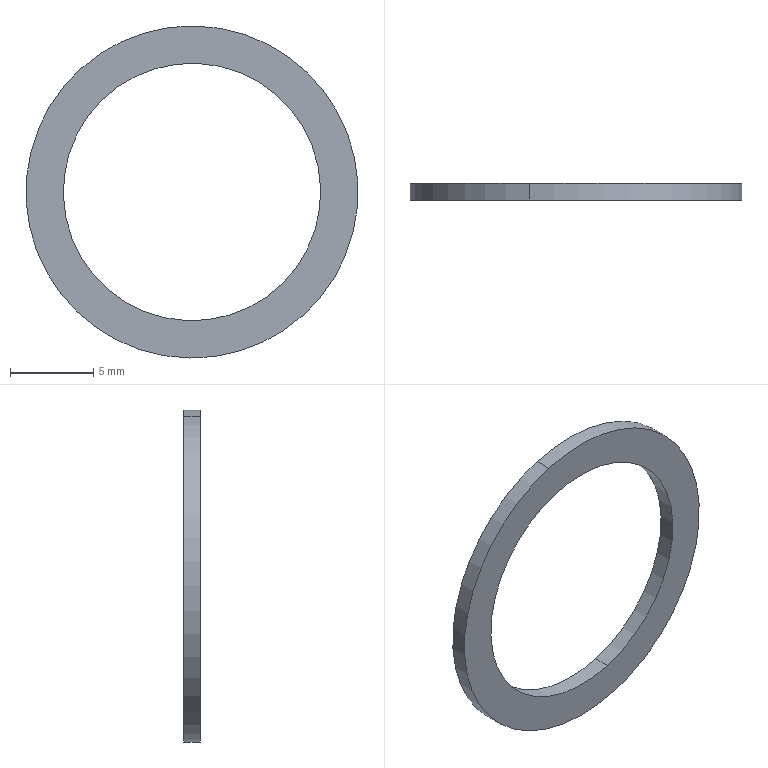Part | SolidWorks | features BaseBody 1 | 1 solid | 6 faces | box 20 x 1 x 20 mm | volume 125.467 mm3 | cylinder 4 | plane 2 | commonest cylinder face diameters 15.5 x2 20 x2
STEP:
#1=CARTESIAN_POINT('',(-385.349,-96.,36.032));
#2=VERTEX_POINT('',#1);
#3=CARTESIAN_POINT('',(-389.7,-96.,50.909));
#4=VERTEX_POINT('',#3);
#5=CARTESIAN_POINT('',(-387.524,-96.,43.47));
#6=DIRECTION('',(0.,-1.,0.));
#7=DIRECTION('',(0.2807,0.,-0.9598));
#8=AXIS2_PLACEMENT_3D('',#5,#6,#7);
#9=CIRCLE('',#8,7.75);
#10=EDGE_CURVE('',#2,#4,#9,.T.);
#11=ORIENTED_EDGE('',*,*,#10,.F.);
#12=CARTESIAN_POINT('',(-385.349,-97.,36.032));
#13=VERTEX_POINT('',#12);
#14=CARTESIAN_POINT('',(-385.349,-96.,36.032));
#15=DIRECTION('',(0.,-1.,0.));
#16=VECTOR('',#15,1000.);
#17=LINE('',#14,#16);
#18=EDGE_CURVE('',#2,#13,#17,.T.);
#19=ORIENTED_EDGE('',*,*,#18,.T.);
#20=CARTESIAN_POINT('',(-389.7,-97.,50.909));
#21=VERTEX_POINT('',#20);
#22=CARTESIAN_POINT('',(-387.524,-97.,43.47));
#23=DIRECTION('',(0.,1.,0.));
#24=DIRECTION('',(-0.2807,0.,0.9598));
#25=AXIS2_PLACEMENT_3D('',#22,#23,#24);
#26=CIRCLE('',#25,7.75);
#27=EDGE_CURVE('',#21,#13,#26,.T.);
#28=ORIENTED_EDGE('',*,*,#27,.F.);
#29=CARTESIAN_POINT('',(-389.7,-96.,50.909));
#30=DIRECTION('',(0.,-1.,0.));
#31=VECTOR('',#30,1000.);
#32=LINE('',#29,#31);
#33=EDGE_CURVE('',#4,#21,#32,.T.);
#34=ORIENTED_EDGE('',*,*,#33,.F.);
#35=EDGE_LOOP('',(#11,#19,#28,#34));
#36=FACE_OUTER_BOUND('',#35,.T.);
#37=CARTESIAN_POINT('',(-387.524,-96.,43.47));
#38=DIRECTION('',(0.,-1.,0.));
#39=DIRECTION('',(-0.2807,0.,0.9598));
#40=AXIS2_PLACEMENT_3D('',#37,#38,#39);
#41=CYLINDRICAL_SURFACE('',#40,7.75);
#42=ADVANCED_FACE('',(#36),#41,.F.);
#43=CARTESIAN_POINT('',(-384.718,-96.,33.872));
#44=VERTEX_POINT('',#43);
#45=CARTESIAN_POINT('',(-390.331,-96.,53.068));
#46=VERTEX_POINT('',#45);
#47=CARTESIAN_POINT('',(-387.524,-96.,43.47));
#48=DIRECTION('',(0.,1.,0.));
#49=DIRECTION('',(-0.2807,0.,0.9598));
#50=AXIS2_PLACEMENT_3D('',#47,#48,#49);
#51=CIRCLE('',#50,10.);
#52=EDGE_CURVE('',#44,#46,#51,.T.);
#53=ORIENTED_EDGE('',*,*,#52,.F.);
#54=CARTESIAN_POINT('',(-384.718,-97.,33.872));
#55=VERTEX_POINT('',#54);
#56=CARTESIAN_POINT('',(-384.718,-96.,33.872));
#57=DIRECTION('',(0.,-1.,0.));
#58=VECTOR('',#57,1000.);
#59=LINE('',#56,#58);
#60=EDGE_CURVE('',#44,#55,#59,.T.);
#61=ORIENTED_EDGE('',*,*,#60,.T.);
#62=CARTESIAN_POINT('',(-390.331,-97.,53.068));
#63=VERTEX_POINT('',#62);
#64=CARTESIAN_POINT('',(-387.524,-97.,43.47));
#65=DIRECTION('',(0.,-1.,0.));
#66=DIRECTION('',(0.2807,0.,-0.9598));
#67=AXIS2_PLACEMENT_3D('',#64,#65,#66);
#68=CIRCLE('',#67,10.);
#69=EDGE_CURVE('',#63,#55,#68,.T.);
#70=ORIENTED_EDGE('',*,*,#69,.F.);
#71=CARTESIAN_POINT('',(-390.331,-96.,53.068));
#72=DIRECTION('',(0.,-1.,0.));
#73=VECTOR('',#72,1000.);
#74=LINE('',#71,#73);
#75=EDGE_CURVE('',#46,#63,#74,.T.);
#76=ORIENTED_EDGE('',*,*,#75,.F.);
#77=EDGE_LOOP('',(#53,#61,#70,#76));
#78=FACE_OUTER_BOUND('',#77,.T.);
#79=CARTESIAN_POINT('',(-387.524,-96.,43.47));
#80=DIRECTION('',(0.,-1.,0.));
#81=DIRECTION('',(-0.2807,0.,0.9598));
#82=AXIS2_PLACEMENT_3D('',#79,#80,#81);
#83=CYLINDRICAL_SURFACE('',#82,10.);
#84=ADVANCED_FACE('',(#78),#83,.T.);
#85=CARTESIAN_POINT('',(-387.524,-96.,43.47));
#86=DIRECTION('',(0.,-1.,0.));
#87=DIRECTION('',(0.2807,0.,-0.9598));
#88=AXIS2_PLACEMENT_3D('',#85,#86,#87);
#89=CIRCLE('',#88,7.75);
#90=EDGE_CURVE('',#4,#2,#89,.T.);
#91=ORIENTED_EDGE('',*,*,#90,.T.);
#92=ORIENTED_EDGE('',*,*,#10,.T.);
#93=EDGE_LOOP('',(#91,#92));
#94=FACE_BOUND('',#93,.T.);
#95=CARTESIAN_POINT('',(-387.524,-96.,43.47));
#96=DIRECTION('',(0.,1.,0.));
#97=DIRECTION('',(-0.2807,0.,0.9598));
#98=AXIS2_PLACEMENT_3D('',#95,#96,#97);
#99=CIRCLE('',#98,10.);
#100=EDGE_CURVE('',#46,#44,#99,.T.);
#101=ORIENTED_EDGE('',*,*,#100,.T.);
#102=ORIENTED_EDGE('',*,*,#52,.T.);
#103=EDGE_LOOP('',(#101,#102));
#104=FACE_OUTER_BOUND('',#103,.T.);
#105=CARTESIAN_POINT('',(-387.524,-96.,43.47));
#106=DIRECTION('',(0.,1.,0.));
#107=DIRECTION('',(1.,0.,0.));
#108=AXIS2_PLACEMENT_3D('',#105,#106,#107);
#109=PLANE('',#108);
#110=ADVANCED_FACE('',(#94,#104),#109,.T.);
#111=ORIENTED_EDGE('',*,*,#60,.F.);
#112=ORIENTED_EDGE('',*,*,#100,.F.);
#113=ORIENTED_EDGE('',*,*,#75,.T.);
#114=CARTESIAN_POINT('',(-387.524,-97.,43.47));
#115=DIRECTION('',(0.,-1.,0.));
#116=DIRECTION('',(0.2807,0.,-0.9598));
#117=AXIS2_PLACEMENT_3D('',#114,#115,#116);
#118=CIRCLE('',#117,10.);
#119=EDGE_CURVE('',#55,#63,#118,.T.);
#120=ORIENTED_EDGE('',*,*,#119,.F.);
#121=EDGE_LOOP('',(#111,#112,#113,#120));
#122=FACE_OUTER_BOUND('',#121,.T.);
#123=CARTESIAN_POINT('',(-387.524,-96.,43.47));
#124=DIRECTION('',(0.,-1.,0.));
#125=DIRECTION('',(-0.2807,0.,0.9598));
#126=AXIS2_PLACEMENT_3D('',#123,#124,#125);
#127=CYLINDRICAL_SURFACE('',#126,10.);
#128=ADVANCED_FACE('',(#122),#127,.T.);
#129=ORIENTED_EDGE('',*,*,#27,.T.);
#130=CARTESIAN_POINT('',(-387.524,-97.,43.47));
#131=DIRECTION('',(0.,1.,0.));
#132=DIRECTION('',(-0.2807,0.,0.9598));
#133=AXIS2_PLACEMENT_3D('',#130,#131,#132);
#134=CIRCLE('',#133,7.75);
#135=EDGE_CURVE('',#13,#21,#134,.T.);
#136=ORIENTED_EDGE('',*,*,#135,.T.);
#137=EDGE_LOOP('',(#129,#136));
#138=FACE_BOUND('',#137,.T.);
#139=ORIENTED_EDGE('',*,*,#69,.T.);
#140=ORIENTED_EDGE('',*,*,#119,.T.);
#141=EDGE_LOOP('',(#139,#140));
#142=FACE_OUTER_BOUND('',#141,.T.);
#143=CARTESIAN_POINT('',(-387.524,-97.,43.47));
#144=DIRECTION('',(0.,1.,0.));
#145=DIRECTION('',(1.,0.,0.));
#146=AXIS2_PLACEMENT_3D('',#143,#144,#145);
#147=PLANE('',#146);
#148=ADVANCED_FACE('',(#138,#142),#147,.F.);
#149=ORIENTED_EDGE('',*,*,#18,.F.);
#150=ORIENTED_EDGE('',*,*,#90,.F.);
#151=ORIENTED_EDGE('',*,*,#33,.T.);
#152=ORIENTED_EDGE('',*,*,#135,.F.);
#153=EDGE_LOOP('',(#149,#150,#151,#152));
#154=FACE_OUTER_BOUND('',#153,.T.);
#155=CARTESIAN_POINT('',(-387.524,-96.,43.47));
#156=DIRECTION('',(0.,-1.,0.));
#157=DIRECTION('',(-0.2807,0.,0.9598));
#158=AXIS2_PLACEMENT_3D('',#155,#156,#157);
#159=CYLINDRICAL_SURFACE('',#158,7.75);
#160=ADVANCED_FACE('',(#154),#159,.F.);
#161=CLOSED_SHELL('',(#42,#84,#110,#128,#148,#160));
#162=MANIFOLD_SOLID_BREP('',#161);
#163=CARTESIAN_POINT('',(0.,0.,0.));
#164=DIRECTION('',(0.,0.,1.));
#165=DIRECTION('',(1.,0.,0.));
#166=AXIS2_PLACEMENT_3D('',#163,#164,#165);
#167=(LENGTH_UNIT()NAMED_UNIT(*)SI_UNIT(.MILLI.,.METRE.));
#168=UNCERTAINTY_MEASURE_WITH_UNIT(LENGTH_MEASURE(0.00001),#167,'','');
#169=(NAMED_UNIT(*)PLANE_ANGLE_UNIT()SI_UNIT($,.RADIAN.));
#170=(NAMED_UNIT(*)SI_UNIT($,.STERADIAN.)SOLID_ANGLE_UNIT());
#171=(GEOMETRIC_REPRESENTATION_CONTEXT(3)GLOBAL_UNCERTAINTY_ASSIGNED_CONTEXT((#168))GLOBAL_UNIT_ASSIGNED_CONTEXT((#167,#169,#170))REPRESENTATION_CONTEXT('',''));
#172=ADVANCED_BREP_SHAPE_REPRESENTATION('',(#162,#166),#171);